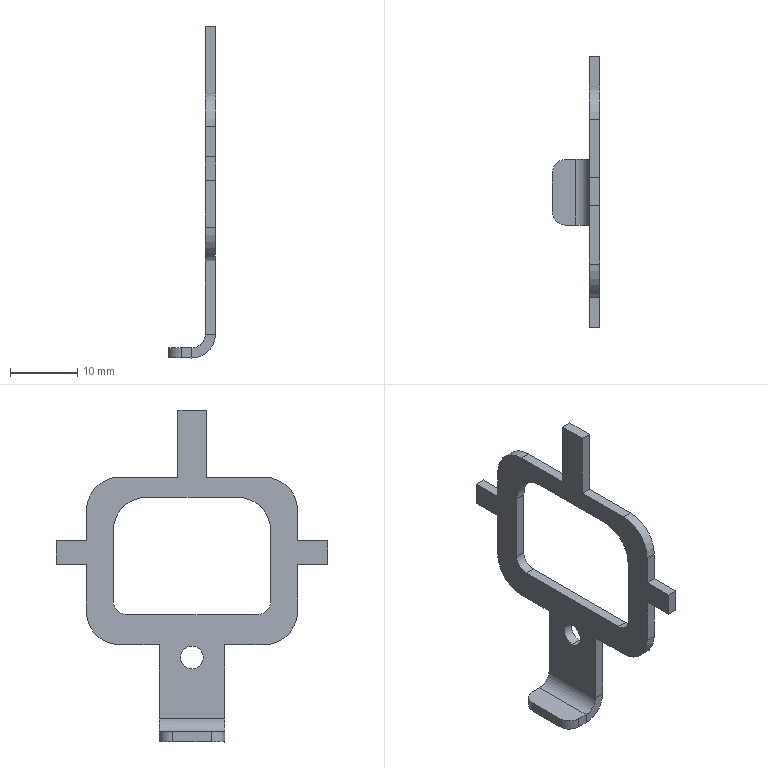Part | SolidWorks | features BaseBody 1 | 1 solid | 46 faces | box 7.041 x 40.502 x 49.501 mm | volume 921.56 mm3 | plane 32 | cylinder 14 | commonest cylinder face diameters 10 x6 4 x5 3.4 x2 7 x1
STEP:
#1=CARTESIAN_POINT('',(-263.159,-4.536,-94.753));
#2=VERTEX_POINT('',#1);
#3=CARTESIAN_POINT('',(-263.16,-4.535,-96.253));
#4=VERTEX_POINT('',#3);
#5=CARTESIAN_POINT('',(-263.159,-4.536,-94.753));
#6=DIRECTION('',(-0.0008339,0.0004454,-1.));
#7=VECTOR('',#6,1000.);
#8=LINE('',#5,#7);
#9=EDGE_CURVE('',#2,#4,#8,.T.);
#10=ORIENTED_EDGE('',*,*,#9,.F.);
#11=CARTESIAN_POINT('',(-261.159,-2.536,-94.754));
#12=VERTEX_POINT('',#11);
#13=CARTESIAN_POINT('',(-261.159,-4.536,-94.755));
#14=DIRECTION('',(-0.0008339,0.0004454,-1.));
#15=DIRECTION('',(-1.,-0.00003864,0.0008339));
#16=AXIS2_PLACEMENT_3D('',#13,#14,#15);
#17=CIRCLE('',#16,2.);
#18=EDGE_CURVE('',#2,#12,#17,.T.);
#19=ORIENTED_EDGE('',*,*,#18,.T.);
#20=CARTESIAN_POINT('',(-261.16,-2.535,-96.254));
#21=VERTEX_POINT('',#20);
#22=CARTESIAN_POINT('',(-261.16,-2.535,-96.254));
#23=DIRECTION('',(0.0008339,-0.0004454,1.));
#24=VECTOR('',#23,1000.);
#25=LINE('',#22,#24);
#26=EDGE_CURVE('',#21,#12,#25,.T.);
#27=ORIENTED_EDGE('',*,*,#26,.F.);
#28=CARTESIAN_POINT('',(-261.16,-4.535,-96.255));
#29=DIRECTION('',(0.0008339,-0.0004454,1.));
#30=DIRECTION('',(-0.00003827,1.,0.0004455));
#31=AXIS2_PLACEMENT_3D('',#28,#29,#30);
#32=CIRCLE('',#31,2.);
#33=EDGE_CURVE('',#21,#4,#32,.T.);
#34=ORIENTED_EDGE('',*,*,#33,.T.);
#35=EDGE_LOOP('',(#10,#19,#27,#34));
#36=FACE_OUTER_BOUND('',#35,.T.);
#37=CARTESIAN_POINT('',(-261.16,-4.535,-96.255));
#38=DIRECTION('',(0.0008339,-0.0004454,1.));
#39=DIRECTION('',(-1.,-0.00003864,0.0008339));
#40=AXIS2_PLACEMENT_3D('',#37,#38,#39);
#41=CYLINDRICAL_SURFACE('',#40,2.);
#42=ADVANCED_FACE('',(#36),#41,.T.);
#43=CARTESIAN_POINT('',(-263.16,-10.335,-96.256));
#44=VERTEX_POINT('',#43);
#45=CARTESIAN_POINT('',(-261.16,-12.335,-96.259));
#46=VERTEX_POINT('',#45);
#47=CARTESIAN_POINT('',(-261.16,-10.335,-96.258));
#48=DIRECTION('',(0.0008339,-0.0004454,1.));
#49=DIRECTION('',(-1.,-0.00003864,0.0008339));
#50=AXIS2_PLACEMENT_3D('',#47,#48,#49);
#51=CIRCLE('',#50,2.);
#52=EDGE_CURVE('',#44,#46,#51,.T.);
#53=ORIENTED_EDGE('',*,*,#52,.F.);
#54=CARTESIAN_POINT('',(-263.16,-4.535,-96.253));
#55=DIRECTION('',(0.00003827,-1.,-0.0004455));
#56=VECTOR('',#55,1000.);
#57=LINE('',#54,#56);
#58=EDGE_CURVE('',#4,#44,#57,.T.);
#59=ORIENTED_EDGE('',*,*,#58,.F.);
#60=ORIENTED_EDGE('',*,*,#33,.F.);
#61=CARTESIAN_POINT('',(-259.66,-2.535,-96.256));
#62=VERTEX_POINT('',#61);
#63=CARTESIAN_POINT('',(-259.66,-2.535,-96.256));
#64=DIRECTION('',(-1.,-0.00003864,0.0008339));
#65=VECTOR('',#64,1000.);
#66=LINE('',#63,#65);
#67=EDGE_CURVE('',#62,#21,#66,.T.);
#68=ORIENTED_EDGE('',*,*,#67,.F.);
#69=CARTESIAN_POINT('',(-259.66,-12.335,-96.26));
#70=VERTEX_POINT('',#69);
#71=CARTESIAN_POINT('',(-259.66,-2.535,-96.256));
#72=DIRECTION('',(0.00003827,-1.,-0.0004455));
#73=VECTOR('',#72,1000.);
#74=LINE('',#71,#73);
#75=EDGE_CURVE('',#62,#70,#74,.T.);
#76=ORIENTED_EDGE('',*,*,#75,.T.);
#77=CARTESIAN_POINT('',(-261.16,-12.335,-96.259));
#78=DIRECTION('',(1.,0.00003864,-0.0008339));
#79=VECTOR('',#78,1000.);
#80=LINE('',#77,#79);
#81=EDGE_CURVE('',#46,#70,#80,.T.);
#82=ORIENTED_EDGE('',*,*,#81,.F.);
#83=EDGE_LOOP('',(#53,#59,#60,#68,#76,#82));
#84=FACE_OUTER_BOUND('',#83,.T.);
#85=CARTESIAN_POINT('',(-257.661,8.315,-96.252));
#86=DIRECTION('',(0.0008339,-0.0004454,1.));
#87=DIRECTION('',(-0.4711,-0.8821,0.));
#88=AXIS2_PLACEMENT_3D('',#85,#86,#87);
#89=PLANE('',#88);
#90=ADVANCED_FACE('',(#84),#89,.F.);
#91=CARTESIAN_POINT('',(-261.159,-12.336,-94.759));
#92=VERTEX_POINT('',#91);
#93=CARTESIAN_POINT('',(-261.159,-12.336,-94.759));
#94=DIRECTION('',(-0.0008339,0.0004454,-1.));
#95=VECTOR('',#94,1000.);
#96=LINE('',#93,#95);
#97=EDGE_CURVE('',#92,#46,#96,.T.);
#98=ORIENTED_EDGE('',*,*,#97,.T.);
#99=ORIENTED_EDGE('',*,*,#81,.T.);
#100=CARTESIAN_POINT('',(-259.659,-12.336,-94.76));
#101=VERTEX_POINT('',#100);
#102=CARTESIAN_POINT('',(-259.66,-12.335,-96.26));
#103=DIRECTION('',(0.0008339,-0.0004454,1.));
#104=VECTOR('',#103,1000.);
#105=LINE('',#102,#104);
#106=EDGE_CURVE('',#70,#101,#105,.T.);
#107=ORIENTED_EDGE('',*,*,#106,.T.);
#108=CARTESIAN_POINT('',(-261.159,-12.336,-94.759));
#109=DIRECTION('',(1.,0.00003864,-0.0008339));
#110=VECTOR('',#109,1000.);
#111=LINE('',#108,#110);
#112=EDGE_CURVE('',#92,#101,#111,.T.);
#113=ORIENTED_EDGE('',*,*,#112,.F.);
#114=EDGE_LOOP('',(#98,#99,#107,#113));
#115=FACE_OUTER_BOUND('',#114,.T.);
#116=CARTESIAN_POINT('',(-263.16,-12.335,-96.257));
#117=DIRECTION('',(-0.00003827,1.,0.0004455));
#118=DIRECTION('',(0.9963,0.,0.08559));
#119=AXIS2_PLACEMENT_3D('',#116,#117,#118);
#120=PLANE('',#119);
#121=ADVANCED_FACE('',(#115),#120,.F.);
#122=CARTESIAN_POINT('',(-263.159,-10.336,-94.756));
#123=VERTEX_POINT('',#122);
#124=CARTESIAN_POINT('',(-261.159,-10.336,-94.758));
#125=DIRECTION('',(-0.0008339,0.0004454,-1.));
#126=DIRECTION('',(0.00003827,-1.,-0.0004455));
#127=AXIS2_PLACEMENT_3D('',#124,#125,#126);
#128=CIRCLE('',#127,2.);
#129=EDGE_CURVE('',#92,#123,#128,.T.);
#130=ORIENTED_EDGE('',*,*,#129,.F.);
#131=ORIENTED_EDGE('',*,*,#112,.T.);
#132=CARTESIAN_POINT('',(-259.659,-2.536,-94.756));
#133=VERTEX_POINT('',#132);
#134=CARTESIAN_POINT('',(-259.659,-12.336,-94.76));
#135=DIRECTION('',(-0.00003827,1.,0.0004455));
#136=VECTOR('',#135,1000.);
#137=LINE('',#134,#136);
#138=EDGE_CURVE('',#101,#133,#137,.T.);
#139=ORIENTED_EDGE('',*,*,#138,.T.);
#140=CARTESIAN_POINT('',(-259.659,-2.536,-94.756));
#141=DIRECTION('',(-1.,-0.00003864,0.0008339));
#142=VECTOR('',#141,1000.);
#143=LINE('',#140,#142);
#144=EDGE_CURVE('',#133,#12,#143,.T.);
#145=ORIENTED_EDGE('',*,*,#144,.T.);
#146=ORIENTED_EDGE('',*,*,#18,.F.);
#147=CARTESIAN_POINT('',(-263.159,-4.536,-94.753));
#148=DIRECTION('',(0.00003827,-1.,-0.0004455));
#149=VECTOR('',#148,1000.);
#150=LINE('',#147,#149);
#151=EDGE_CURVE('',#2,#123,#150,.T.);
#152=ORIENTED_EDGE('',*,*,#151,.T.);
#153=EDGE_LOOP('',(#130,#131,#139,#145,#146,#152));
#154=FACE_OUTER_BOUND('',#153,.T.);
#155=CARTESIAN_POINT('',(-257.66,8.314,-94.752));
#156=DIRECTION('',(0.0008339,-0.0004454,1.));
#157=DIRECTION('',(-0.4711,-0.8821,0.));
#158=AXIS2_PLACEMENT_3D('',#155,#156,#157);
#159=PLANE('',#158);
#160=ADVANCED_FACE('',(#154),#159,.T.);
#161=CARTESIAN_POINT('',(-263.16,-10.335,-96.256));
#162=DIRECTION('',(0.0008339,-0.0004454,1.));
#163=VECTOR('',#162,1000.);
#164=LINE('',#161,#163);
#165=EDGE_CURVE('',#44,#123,#164,.T.);
#166=ORIENTED_EDGE('',*,*,#165,.T.);
#167=ORIENTED_EDGE('',*,*,#151,.F.);
#168=ORIENTED_EDGE('',*,*,#9,.T.);
#169=ORIENTED_EDGE('',*,*,#58,.T.);
#170=EDGE_LOOP('',(#166,#167,#168,#169));
#171=FACE_OUTER_BOUND('',#170,.T.);
#172=CARTESIAN_POINT('',(-263.16,-2.535,-96.253));
#173=DIRECTION('',(1.,0.00003864,-0.0008339));
#174=DIRECTION('',(0.,-0.9989,-0.04628));
#175=AXIS2_PLACEMENT_3D('',#172,#173,#174);
#176=PLANE('',#175);
#177=ADVANCED_FACE('',(#171),#176,.F.);
#178=ORIENTED_EDGE('',*,*,#97,.F.);
#179=ORIENTED_EDGE('',*,*,#129,.T.);
#180=ORIENTED_EDGE('',*,*,#165,.F.);
#181=ORIENTED_EDGE('',*,*,#52,.T.);
#182=EDGE_LOOP('',(#178,#179,#180,#181));
#183=FACE_OUTER_BOUND('',#182,.T.);
#184=CARTESIAN_POINT('',(-261.16,-10.335,-96.258));
#185=DIRECTION('',(0.0008339,-0.0004454,1.));
#186=DIRECTION('',(-1.,-0.00003864,0.0008339));
#187=AXIS2_PLACEMENT_3D('',#184,#185,#186);
#188=CYLINDRICAL_SURFACE('',#187,2.);
#189=ADVANCED_FACE('',(#183),#188,.T.);
#190=ORIENTED_EDGE('',*,*,#26,.T.);
#191=ORIENTED_EDGE('',*,*,#144,.F.);
#192=CARTESIAN_POINT('',(-259.66,-2.535,-96.256));
#193=DIRECTION('',(0.0008339,-0.0004454,1.));
#194=VECTOR('',#193,1000.);
#195=LINE('',#192,#194);
#196=EDGE_CURVE('',#62,#133,#195,.T.);
#197=ORIENTED_EDGE('',*,*,#196,.F.);
#198=ORIENTED_EDGE('',*,*,#67,.T.);
#199=EDGE_LOOP('',(#190,#191,#197,#198));
#200=FACE_OUTER_BOUND('',#199,.T.);
#201=CARTESIAN_POINT('',(-257.66,-2.535,-96.257));
#202=DIRECTION('',(0.00003827,-1.,-0.0004455));
#203=DIRECTION('',(0.,0.0004455,-1.));
#204=AXIS2_PLACEMENT_3D('',#201,#202,#203);
#205=PLANE('',#204);
#206=ADVANCED_FACE('',(#200),#205,.F.);
#207=CARTESIAN_POINT('',(-257.657,-2.537,-92.757));
#208=VERTEX_POINT('',#207);
#209=CARTESIAN_POINT('',(-259.657,-2.537,-92.756));
#210=DIRECTION('',(-0.00003827,1.,0.0004455));
#211=DIRECTION('',(1.,0.00003864,-0.0008339));
#212=AXIS2_PLACEMENT_3D('',#209,#210,#211);
#213=CIRCLE('',#212,2.);
#214=EDGE_CURVE('',#208,#133,#213,.T.);
#215=ORIENTED_EDGE('',*,*,#214,.F.);
#216=CARTESIAN_POINT('',(-256.157,-2.537,-92.758));
#217=VERTEX_POINT('',#216);
#218=CARTESIAN_POINT('',(-256.157,-2.537,-92.758));
#219=DIRECTION('',(-1.,-0.00003864,0.0008339));
#220=VECTOR('',#219,1000.);
#221=LINE('',#218,#220);
#222=EDGE_CURVE('',#217,#208,#221,.T.);
#223=ORIENTED_EDGE('',*,*,#222,.F.);
#224=CARTESIAN_POINT('',(-259.657,-2.537,-92.756));
#225=DIRECTION('',(0.00003827,-1.,-0.0004455));
#226=DIRECTION('',(-0.0008339,0.0004454,-1.));
#227=AXIS2_PLACEMENT_3D('',#224,#225,#226);
#228=CIRCLE('',#227,3.5);
#229=EDGE_CURVE('',#62,#217,#228,.T.);
#230=ORIENTED_EDGE('',*,*,#229,.F.);
#231=ORIENTED_EDGE('',*,*,#196,.T.);
#232=EDGE_LOOP('',(#215,#223,#230,#231));
#233=FACE_OUTER_BOUND('',#232,.T.);
#234=CARTESIAN_POINT('',(-259.657,-2.537,-92.756));
#235=DIRECTION('',(-0.00003827,1.,0.0004455));
#236=DIRECTION('',(0.9963,0.,0.08559));
#237=AXIS2_PLACEMENT_3D('',#234,#235,#236);
#238=PLANE('',#237);
#239=ADVANCED_FACE('',(#233),#238,.T.);
#240=CARTESIAN_POINT('',(-256.157,-12.337,-92.763));
#241=VERTEX_POINT('',#240);
#242=CARTESIAN_POINT('',(-259.657,-12.337,-92.76));
#243=DIRECTION('',(-0.00003827,1.,0.0004455));
#244=DIRECTION('',(1.,0.00003864,-0.0008339));
#245=AXIS2_PLACEMENT_3D('',#242,#243,#244);
#246=CIRCLE('',#245,3.5);
#247=EDGE_CURVE('',#241,#70,#246,.T.);
#248=ORIENTED_EDGE('',*,*,#247,.T.);
#249=ORIENTED_EDGE('',*,*,#75,.F.);
#250=ORIENTED_EDGE('',*,*,#229,.T.);
#251=CARTESIAN_POINT('',(-256.157,-12.337,-92.763));
#252=DIRECTION('',(-0.00003827,1.,0.0004455));
#253=VECTOR('',#252,1000.);
#254=LINE('',#251,#253);
#255=EDGE_CURVE('',#241,#217,#254,.T.);
#256=ORIENTED_EDGE('',*,*,#255,.F.);
#257=EDGE_LOOP('',(#248,#249,#250,#256));
#258=FACE_OUTER_BOUND('',#257,.T.);
#259=CARTESIAN_POINT('',(-259.657,-12.337,-92.76));
#260=DIRECTION('',(0.00003827,-1.,-0.0004455));
#261=DIRECTION('',(-0.0008339,0.0004454,-1.));
#262=AXIS2_PLACEMENT_3D('',#259,#260,#261);
#263=CYLINDRICAL_SURFACE('',#262,3.5);
#264=ADVANCED_FACE('',(#258),#263,.T.);
#265=CARTESIAN_POINT('',(-256.142,-19.194,-75.266));
#266=VERTEX_POINT('',#265);
#267=CARTESIAN_POINT('',(-256.144,-17.193,-77.265));
#268=VERTEX_POINT('',#267);
#269=CARTESIAN_POINT('',(-256.142,-17.194,-75.265));
#270=DIRECTION('',(1.,0.00003864,-0.0008339));
#271=DIRECTION('',(0.00003827,-1.,-0.0004455));
#272=AXIS2_PLACEMENT_3D('',#269,#270,#271);
#273=CIRCLE('',#272,2.);
#274=EDGE_CURVE('',#266,#268,#273,.T.);
#275=ORIENTED_EDGE('',*,*,#274,.F.);
#276=CARTESIAN_POINT('',(-256.133,-19.199,-64.766));
#277=VERTEX_POINT('',#276);
#278=CARTESIAN_POINT('',(-256.133,-19.199,-64.766));
#279=DIRECTION('',(-0.0008339,0.0004454,-1.));
#280=VECTOR('',#279,1000.);
#281=LINE('',#278,#280);
#282=EDGE_CURVE('',#277,#266,#281,.T.);
#283=ORIENTED_EDGE('',*,*,#282,.F.);
#284=CARTESIAN_POINT('',(-256.129,-14.201,-59.764));
#285=VERTEX_POINT('',#284);
#286=CARTESIAN_POINT('',(-256.134,-14.199,-64.764));
#287=DIRECTION('',(1.,0.00003864,-0.0008339));
#288=DIRECTION('',(0.0008339,-0.0004454,1.));
#289=AXIS2_PLACEMENT_3D('',#286,#287,#288);
#290=CIRCLE('',#289,5.);
#291=EDGE_CURVE('',#285,#277,#290,.T.);
#292=ORIENTED_EDGE('',*,*,#291,.F.);
#293=CARTESIAN_POINT('',(-256.13,-0.7013,-59.758));
#294=VERTEX_POINT('',#293);
#295=CARTESIAN_POINT('',(-256.13,-0.7013,-59.758));
#296=DIRECTION('',(0.00003827,-1.,-0.0004455));
#297=VECTOR('',#296,1000.);
#298=LINE('',#295,#297);
#299=EDGE_CURVE('',#294,#285,#298,.T.);
#300=ORIENTED_EDGE('',*,*,#299,.F.);
#301=CARTESIAN_POINT('',(-256.134,4.301,-64.755));
#302=VERTEX_POINT('',#301);
#303=CARTESIAN_POINT('',(-256.134,-0.699,-64.758));
#304=DIRECTION('',(1.,0.00003864,-0.0008339));
#305=DIRECTION('',(-0.00003827,1.,0.0004455));
#306=AXIS2_PLACEMENT_3D('',#303,#304,#305);
#307=CIRCLE('',#306,5.);
#308=EDGE_CURVE('',#302,#294,#307,.T.);
#309=ORIENTED_EDGE('',*,*,#308,.F.);
#310=CARTESIAN_POINT('',(-256.143,4.306,-75.255));
#311=VERTEX_POINT('',#310);
#312=CARTESIAN_POINT('',(-256.143,4.306,-75.255));
#313=DIRECTION('',(0.0008339,-0.0004454,1.));
#314=VECTOR('',#313,1000.);
#315=LINE('',#312,#314);
#316=EDGE_CURVE('',#311,#302,#315,.T.);
#317=ORIENTED_EDGE('',*,*,#316,.F.);
#318=CARTESIAN_POINT('',(-256.145,2.307,-77.256));
#319=VERTEX_POINT('',#318);
#320=CARTESIAN_POINT('',(-256.143,2.306,-75.256));
#321=DIRECTION('',(1.,0.00003864,-0.0008339));
#322=DIRECTION('',(-0.0008339,0.0004454,-1.));
#323=AXIS2_PLACEMENT_3D('',#320,#321,#322);
#324=CIRCLE('',#323,2.);
#325=EDGE_CURVE('',#319,#311,#324,.T.);
#326=ORIENTED_EDGE('',*,*,#325,.F.);
#327=CARTESIAN_POINT('',(-256.144,-17.193,-77.265));
#328=DIRECTION('',(-0.00003827,1.,0.0004455));
#329=VECTOR('',#328,1000.);
#330=LINE('',#327,#329);
#331=EDGE_CURVE('',#268,#319,#330,.T.);
#332=ORIENTED_EDGE('',*,*,#331,.F.);
#333=EDGE_LOOP('',(#275,#283,#292,#300,#309,#317,#326,#332));
#334=FACE_BOUND('',#333,.T.);
#335=CARTESIAN_POINT('',(-256.148,-7.441,-81.961));
#336=VERTEX_POINT('',#335);
#337=CARTESIAN_POINT('',(-256.151,-7.44,-85.361));
#338=VERTEX_POINT('',#337);
#339=CARTESIAN_POINT('',(-256.15,-7.441,-83.661));
#340=DIRECTION('',(1.,0.00003864,-0.0008339));
#341=DIRECTION('',(0.0008339,-0.0004454,1.));
#342=AXIS2_PLACEMENT_3D('',#339,#340,#341);
#343=CIRCLE('',#342,1.7);
#344=EDGE_CURVE('',#336,#338,#343,.T.);
#345=ORIENTED_EDGE('',*,*,#344,.F.);
#346=CARTESIAN_POINT('',(-256.15,-7.441,-83.661));
#347=DIRECTION('',(1.,0.00003864,-0.0008339));
#348=DIRECTION('',(-0.0008339,0.0004454,-1.));
#349=AXIS2_PLACEMENT_3D('',#346,#347,#348);
#350=CIRCLE('',#349,1.7);
#351=EDGE_CURVE('',#338,#336,#350,.T.);
#352=ORIENTED_EDGE('',*,*,#351,.F.);
#353=EDGE_LOOP('',(#345,#352));
#354=FACE_BOUND('',#353,.T.);
#355=ORIENTED_EDGE('',*,*,#255,.T.);
#356=CARTESIAN_POINT('',(-256.148,-2.541,-81.758));
#357=VERTEX_POINT('',#356);
#358=CARTESIAN_POINT('',(-256.157,-2.537,-92.758));
#359=DIRECTION('',(0.0008339,-0.0004454,1.));
#360=VECTOR('',#359,1000.);
#361=LINE('',#358,#360);
#362=EDGE_CURVE('',#217,#357,#361,.T.);
#363=ORIENTED_EDGE('',*,*,#362,.T.);
#364=CARTESIAN_POINT('',(-256.148,3.309,-81.756));
#365=VERTEX_POINT('',#364);
#366=CARTESIAN_POINT('',(-256.148,-2.541,-81.758));
#367=DIRECTION('',(-0.00003827,1.,0.0004455));
#368=VECTOR('',#367,1000.);
#369=LINE('',#366,#368);
#370=EDGE_CURVE('',#357,#365,#369,.T.);
#371=ORIENTED_EDGE('',*,*,#370,.T.);
#372=CARTESIAN_POINT('',(-256.145,8.306,-76.754));
#373=VERTEX_POINT('',#372);
#374=CARTESIAN_POINT('',(-256.144,3.306,-76.756));
#375=DIRECTION('',(-1.,-0.00003864,0.0008339));
#376=DIRECTION('',(-0.00003827,1.,0.0004455));
#377=AXIS2_PLACEMENT_3D('',#374,#375,#376);
#378=CIRCLE('',#377,5.);
#379=EDGE_CURVE('',#373,#365,#378,.T.);
#380=ORIENTED_EDGE('',*,*,#379,.F.);
#381=CARTESIAN_POINT('',(-256.139,8.303,-69.754));
#382=VERTEX_POINT('',#381);
#383=CARTESIAN_POINT('',(-256.145,8.306,-76.754));
#384=DIRECTION('',(0.0008339,-0.0004454,1.));
#385=VECTOR('',#384,1000.);
#386=LINE('',#383,#385);
#387=EDGE_CURVE('',#373,#382,#386,.T.);
#388=ORIENTED_EDGE('',*,*,#387,.T.);
#389=CARTESIAN_POINT('',(-256.139,12.803,-69.752));
#390=VERTEX_POINT('',#389);
#391=CARTESIAN_POINT('',(-256.139,8.303,-69.754));
#392=DIRECTION('',(-0.00003827,1.,0.0004455));
#393=VECTOR('',#392,1000.);
#394=LINE('',#391,#393);
#395=EDGE_CURVE('',#382,#390,#394,.T.);
#396=ORIENTED_EDGE('',*,*,#395,.T.);
#397=CARTESIAN_POINT('',(-256.136,12.802,-66.252));
#398=VERTEX_POINT('',#397);
#399=CARTESIAN_POINT('',(-256.139,12.803,-69.752));
#400=DIRECTION('',(0.0008339,-0.0004454,1.));
#401=VECTOR('',#400,1000.);
#402=LINE('',#399,#401);
#403=EDGE_CURVE('',#390,#398,#402,.T.);
#404=ORIENTED_EDGE('',*,*,#403,.T.);
#405=CARTESIAN_POINT('',(-256.136,8.302,-66.254));
#406=VERTEX_POINT('',#405);
#407=CARTESIAN_POINT('',(-256.136,12.802,-66.252));
#408=DIRECTION('',(0.00003827,-1.,-0.0004455));
#409=VECTOR('',#408,1000.);
#410=LINE('',#407,#409);
#411=EDGE_CURVE('',#398,#406,#410,.T.);
#412=ORIENTED_EDGE('',*,*,#411,.T.);
#413=CARTESIAN_POINT('',(-256.132,8.3,-61.754));
#414=VERTEX_POINT('',#413);
#415=CARTESIAN_POINT('',(-256.136,8.302,-66.254));
#416=DIRECTION('',(0.0008339,-0.0004454,1.));
#417=VECTOR('',#416,1000.);
#418=LINE('',#415,#417);
#419=EDGE_CURVE('',#406,#414,#418,.T.);
#420=ORIENTED_EDGE('',*,*,#419,.T.);
#421=CARTESIAN_POINT('',(-256.128,3.297,-56.756));
#422=VERTEX_POINT('',#421);
#423=CARTESIAN_POINT('',(-256.132,3.3,-61.756));
#424=DIRECTION('',(-1.,-0.00003864,0.0008339));
#425=DIRECTION('',(0.0008339,-0.0004454,1.));
#426=AXIS2_PLACEMENT_3D('',#423,#424,#425);
#427=CIRCLE('',#426,5.);
#428=EDGE_CURVE('',#422,#414,#427,.T.);
#429=ORIENTED_EDGE('',*,*,#428,.F.);
#430=CARTESIAN_POINT('',(-256.127,-5.353,-56.76));
#431=VERTEX_POINT('',#430);
#432=CARTESIAN_POINT('',(-256.128,3.297,-56.756));
#433=DIRECTION('',(0.00003827,-1.,-0.0004455));
#434=VECTOR('',#433,1000.);
#435=LINE('',#432,#434);
#436=EDGE_CURVE('',#422,#431,#435,.T.);
#437=ORIENTED_EDGE('',*,*,#436,.T.);
#438=CARTESIAN_POINT('',(-256.119,-5.357,-46.76));
#439=VERTEX_POINT('',#438);
#440=CARTESIAN_POINT('',(-256.127,-5.353,-56.76));
#441=DIRECTION('',(0.0008339,-0.0004454,1.));
#442=VECTOR('',#441,1000.);
#443=LINE('',#440,#442);
#444=EDGE_CURVE('',#431,#439,#443,.T.);
#445=ORIENTED_EDGE('',*,*,#444,.T.);
#446=CARTESIAN_POINT('',(-256.119,-9.557,-46.762));
#447=VERTEX_POINT('',#446);
#448=CARTESIAN_POINT('',(-256.119,-5.357,-46.76));
#449=DIRECTION('',(0.00003827,-1.,-0.0004455));
#450=VECTOR('',#449,1000.);
#451=LINE('',#448,#450);
#452=EDGE_CURVE('',#439,#447,#451,.T.);
#453=ORIENTED_EDGE('',*,*,#452,.T.);
#454=CARTESIAN_POINT('',(-256.127,-9.553,-56.762));
#455=VERTEX_POINT('',#454);
#456=CARTESIAN_POINT('',(-256.119,-9.557,-46.762));
#457=DIRECTION('',(-0.0008339,0.0004454,-1.));
#458=VECTOR('',#457,1000.);
#459=LINE('',#456,#458);
#460=EDGE_CURVE('',#447,#455,#459,.T.);
#461=ORIENTED_EDGE('',*,*,#460,.T.);
#462=CARTESIAN_POINT('',(-256.127,-18.203,-56.765));
#463=VERTEX_POINT('',#462);
#464=CARTESIAN_POINT('',(-256.127,-9.553,-56.762));
#465=DIRECTION('',(0.00003827,-1.,-0.0004455));
#466=VECTOR('',#465,1000.);
#467=LINE('',#464,#466);
#468=EDGE_CURVE('',#455,#463,#467,.T.);
#469=ORIENTED_EDGE('',*,*,#468,.T.);
#470=CARTESIAN_POINT('',(-256.131,-23.2,-61.768));
#471=VERTEX_POINT('',#470);
#472=CARTESIAN_POINT('',(-256.131,-18.2,-61.765));
#473=DIRECTION('',(-1.,-0.00003864,0.0008339));
#474=DIRECTION('',(0.00003827,-1.,-0.0004455));
#475=AXIS2_PLACEMENT_3D('',#472,#473,#474);
#476=CIRCLE('',#475,5.);
#477=EDGE_CURVE('',#471,#463,#476,.T.);
#478=ORIENTED_EDGE('',*,*,#477,.F.);
#479=CARTESIAN_POINT('',(-256.135,-23.198,-66.268));
#480=VERTEX_POINT('',#479);
#481=CARTESIAN_POINT('',(-256.131,-23.2,-61.768));
#482=DIRECTION('',(-0.0008339,0.0004454,-1.));
#483=VECTOR('',#482,1000.);
#484=LINE('',#481,#483);
#485=EDGE_CURVE('',#471,#480,#484,.T.);
#486=ORIENTED_EDGE('',*,*,#485,.T.);
#487=CARTESIAN_POINT('',(-256.134,-27.698,-66.27));
#488=VERTEX_POINT('',#487);
#489=CARTESIAN_POINT('',(-256.135,-23.198,-66.268));
#490=DIRECTION('',(0.00003827,-1.,-0.0004455));
#491=VECTOR('',#490,1000.);
#492=LINE('',#489,#491);
#493=EDGE_CURVE('',#480,#488,#492,.T.);
#494=ORIENTED_EDGE('',*,*,#493,.T.);
#495=CARTESIAN_POINT('',(-256.137,-27.697,-69.77));
#496=VERTEX_POINT('',#495);
#497=CARTESIAN_POINT('',(-256.134,-27.698,-66.27));
#498=DIRECTION('',(-0.0008339,0.0004454,-1.));
#499=VECTOR('',#498,1000.);
#500=LINE('',#497,#499);
#501=EDGE_CURVE('',#488,#496,#500,.T.);
#502=ORIENTED_EDGE('',*,*,#501,.T.);
#503=CARTESIAN_POINT('',(-256.137,-23.197,-69.768));
#504=VERTEX_POINT('',#503);
#505=CARTESIAN_POINT('',(-256.137,-27.697,-69.77));
#506=DIRECTION('',(-0.00003827,1.,0.0004455));
#507=VECTOR('',#506,1000.);
#508=LINE('',#505,#507);
#509=EDGE_CURVE('',#496,#504,#508,.T.);
#510=ORIENTED_EDGE('',*,*,#509,.T.);
#511=CARTESIAN_POINT('',(-256.143,-23.194,-76.768));
#512=VERTEX_POINT('',#511);
#513=CARTESIAN_POINT('',(-256.137,-23.197,-69.768));
#514=DIRECTION('',(-0.0008339,0.0004454,-1.));
#515=VECTOR('',#514,1000.);
#516=LINE('',#513,#515);
#517=EDGE_CURVE('',#504,#512,#516,.T.);
#518=ORIENTED_EDGE('',*,*,#517,.T.);
#519=CARTESIAN_POINT('',(-256.148,-18.191,-81.765));
#520=VERTEX_POINT('',#519);
#521=CARTESIAN_POINT('',(-256.143,-18.194,-76.765));
#522=DIRECTION('',(-1.,-0.00003864,0.0008339));
#523=DIRECTION('',(-0.0008339,0.0004454,-1.));
#524=AXIS2_PLACEMENT_3D('',#521,#522,#523);
#525=CIRCLE('',#524,5.);
#526=EDGE_CURVE('',#520,#512,#525,.T.);
#527=ORIENTED_EDGE('',*,*,#526,.F.);
#528=CARTESIAN_POINT('',(-256.148,-12.341,-81.763));
#529=VERTEX_POINT('',#528);
#530=CARTESIAN_POINT('',(-256.148,-18.191,-81.765));
#531=DIRECTION('',(-0.00003827,1.,0.0004455));
#532=VECTOR('',#531,1000.);
#533=LINE('',#530,#532);
#534=EDGE_CURVE('',#520,#529,#533,.T.);
#535=ORIENTED_EDGE('',*,*,#534,.T.);
#536=CARTESIAN_POINT('',(-256.148,-12.341,-81.763));
#537=DIRECTION('',(-0.0008339,0.0004454,-1.));
#538=VECTOR('',#537,1000.);
#539=LINE('',#536,#538);
#540=EDGE_CURVE('',#529,#241,#539,.T.);
#541=ORIENTED_EDGE('',*,*,#540,.T.);
#542=EDGE_LOOP('',(#355,#363,#371,#380,#388,#396,#404,#412,#420,#429,#437,#445,#453,#461,#469,#478,#486,#494,#502,#510,#518,#527,#535,#541));
#543=FACE_OUTER_BOUND('',#542,.T.);
#544=CARTESIAN_POINT('',(-256.128,8.297,-56.754));
#545=DIRECTION('',(1.,0.00003864,-0.0008339));
#546=DIRECTION('',(0.,-0.9989,-0.04628));
#547=AXIS2_PLACEMENT_3D('',#544,#545,#546);
#548=PLANE('',#547);
#549=ADVANCED_FACE('',(#334,#354,#543),#548,.T.);
#550=CARTESIAN_POINT('',(-257.657,-12.337,-92.762));
#551=VERTEX_POINT('',#550);
#552=CARTESIAN_POINT('',(-256.157,-12.337,-92.763));
#553=DIRECTION('',(-1.,-0.00003864,0.0008339));
#554=VECTOR('',#553,1000.);
#555=LINE('',#552,#554);
#556=EDGE_CURVE('',#241,#551,#555,.T.);
#557=ORIENTED_EDGE('',*,*,#556,.F.);
#558=ORIENTED_EDGE('',*,*,#540,.F.);
#559=CARTESIAN_POINT('',(-257.648,-12.342,-81.762));
#560=VERTEX_POINT('',#559);
#561=CARTESIAN_POINT('',(-257.648,-12.342,-81.762));
#562=DIRECTION('',(1.,0.00003864,-0.0008339));
#563=VECTOR('',#562,1000.);
#564=LINE('',#561,#563);
#565=EDGE_CURVE('',#560,#529,#564,.T.);
#566=ORIENTED_EDGE('',*,*,#565,.F.);
#567=CARTESIAN_POINT('',(-257.648,-12.342,-81.762));
#568=DIRECTION('',(-0.0008339,0.0004454,-1.));
#569=VECTOR('',#568,1000.);
#570=LINE('',#567,#569);
#571=EDGE_CURVE('',#560,#551,#570,.T.);
#572=ORIENTED_EDGE('',*,*,#571,.T.);
#573=EDGE_LOOP('',(#557,#558,#566,#572));
#574=FACE_OUTER_BOUND('',#573,.T.);
#575=CARTESIAN_POINT('',(-256.148,-12.341,-81.763));
#576=DIRECTION('',(0.00003827,-1.,-0.0004455));
#577=DIRECTION('',(0.,0.0004455,-1.));
#578=AXIS2_PLACEMENT_3D('',#575,#576,#577);
#579=PLANE('',#578);
#580=ADVANCED_FACE('',(#574),#579,.T.);
#581=CARTESIAN_POINT('',(-257.63,-0.7013,-59.756));
#582=VERTEX_POINT('',#581);
#583=CARTESIAN_POINT('',(-257.634,4.301,-64.754));
#584=VERTEX_POINT('',#583);
#585=CARTESIAN_POINT('',(-257.634,-0.6991,-64.756));
#586=DIRECTION('',(-1.,-0.00003864,0.0008339));
#587=DIRECTION('',(0.0008339,-0.0004454,1.));
#588=AXIS2_PLACEMENT_3D('',#585,#586,#587);
#589=CIRCLE('',#588,5.);
#590=EDGE_CURVE('',#582,#584,#589,.T.);
#591=ORIENTED_EDGE('',*,*,#590,.F.);
#592=CARTESIAN_POINT('',(-257.629,-14.201,-59.762));
#593=VERTEX_POINT('',#592);
#594=CARTESIAN_POINT('',(-257.63,-0.7013,-59.756));
#595=DIRECTION('',(0.00003827,-1.,-0.0004455));
#596=VECTOR('',#595,1000.);
#597=LINE('',#594,#596);
#598=EDGE_CURVE('',#582,#593,#597,.T.);
#599=ORIENTED_EDGE('',*,*,#598,.T.);
#600=CARTESIAN_POINT('',(-257.633,-19.199,-64.765));
#601=VERTEX_POINT('',#600);
#602=CARTESIAN_POINT('',(-257.634,-14.199,-64.762));
#603=DIRECTION('',(-1.,-0.00003864,0.0008339));
#604=DIRECTION('',(0.00003827,-1.,-0.0004455));
#605=AXIS2_PLACEMENT_3D('',#602,#603,#604);
#606=CIRCLE('',#605,5.);
#607=EDGE_CURVE('',#601,#593,#606,.T.);
#608=ORIENTED_EDGE('',*,*,#607,.F.);
#609=CARTESIAN_POINT('',(-257.642,-19.194,-75.265));
#610=VERTEX_POINT('',#609);
#611=CARTESIAN_POINT('',(-257.633,-19.199,-64.765));
#612=DIRECTION('',(-0.0008339,0.0004454,-1.));
#613=VECTOR('',#612,1000.);
#614=LINE('',#611,#613);
#615=EDGE_CURVE('',#601,#610,#614,.T.);
#616=ORIENTED_EDGE('',*,*,#615,.T.);
#617=CARTESIAN_POINT('',(-257.644,-17.194,-77.264));
#618=VERTEX_POINT('',#617);
#619=CARTESIAN_POINT('',(-257.642,-17.194,-75.264));
#620=DIRECTION('',(-1.,-0.00003864,0.0008339));
#621=DIRECTION('',(-0.0008339,0.0004454,-1.));
#622=AXIS2_PLACEMENT_3D('',#619,#620,#621);
#623=CIRCLE('',#622,2.);
#624=EDGE_CURVE('',#618,#610,#623,.T.);
#625=ORIENTED_EDGE('',*,*,#624,.F.);
#626=CARTESIAN_POINT('',(-257.645,2.306,-77.255));
#627=VERTEX_POINT('',#626);
#628=CARTESIAN_POINT('',(-257.644,-17.194,-77.264));
#629=DIRECTION('',(-0.00003827,1.,0.0004455));
#630=VECTOR('',#629,1000.);
#631=LINE('',#628,#630);
#632=EDGE_CURVE('',#618,#627,#631,.T.);
#633=ORIENTED_EDGE('',*,*,#632,.T.);
#634=CARTESIAN_POINT('',(-257.643,4.306,-75.254));
#635=VERTEX_POINT('',#634);
#636=CARTESIAN_POINT('',(-257.643,2.306,-75.255));
#637=DIRECTION('',(-1.,-0.00003864,0.0008339));
#638=DIRECTION('',(-0.00003827,1.,0.0004455));
#639=AXIS2_PLACEMENT_3D('',#636,#637,#638);
#640=CIRCLE('',#639,2.);
#641=EDGE_CURVE('',#635,#627,#640,.T.);
#642=ORIENTED_EDGE('',*,*,#641,.F.);
#643=CARTESIAN_POINT('',(-257.643,4.306,-75.254));
#644=DIRECTION('',(0.0008339,-0.0004454,1.));
#645=VECTOR('',#644,1000.);
#646=LINE('',#643,#645);
#647=EDGE_CURVE('',#635,#584,#646,.T.);
#648=ORIENTED_EDGE('',*,*,#647,.T.);
#649=EDGE_LOOP('',(#591,#599,#608,#616,#625,#633,#642,#648));
#650=FACE_BOUND('',#649,.T.);
#651=CARTESIAN_POINT('',(-257.648,-7.441,-81.959));
#652=VERTEX_POINT('',#651);
#653=CARTESIAN_POINT('',(-257.651,-7.44,-85.359));
#654=VERTEX_POINT('',#653);
#655=CARTESIAN_POINT('',(-257.65,-7.441,-83.659));
#656=DIRECTION('',(-1.,-0.00003864,0.0008339));
#657=DIRECTION('',(0.0008339,-0.0004454,1.));
#658=AXIS2_PLACEMENT_3D('',#655,#656,#657);
#659=CIRCLE('',#658,1.7);
#660=EDGE_CURVE('',#652,#654,#659,.T.);
#661=ORIENTED_EDGE('',*,*,#660,.F.);
#662=CARTESIAN_POINT('',(-257.65,-7.441,-83.659));
#663=DIRECTION('',(-1.,-0.00003864,0.0008339));
#664=DIRECTION('',(-0.0008339,0.0004454,-1.));
#665=AXIS2_PLACEMENT_3D('',#662,#663,#664);
#666=CIRCLE('',#665,1.7);
#667=EDGE_CURVE('',#654,#652,#666,.T.);
#668=ORIENTED_EDGE('',*,*,#667,.F.);
#669=EDGE_LOOP('',(#661,#668));
#670=FACE_BOUND('',#669,.T.);
#671=ORIENTED_EDGE('',*,*,#571,.F.);
#672=CARTESIAN_POINT('',(-257.648,-18.192,-81.764));
#673=VERTEX_POINT('',#672);
#674=CARTESIAN_POINT('',(-257.648,-18.192,-81.764));
#675=DIRECTION('',(-0.00003827,1.,0.0004455));
#676=VECTOR('',#675,1000.);
#677=LINE('',#674,#676);
#678=EDGE_CURVE('',#673,#560,#677,.T.);
#679=ORIENTED_EDGE('',*,*,#678,.F.);
#680=CARTESIAN_POINT('',(-257.643,-23.194,-76.766));
#681=VERTEX_POINT('',#680);
#682=CARTESIAN_POINT('',(-257.643,-18.194,-76.764));
#683=DIRECTION('',(1.,0.00003864,-0.0008339));
#684=DIRECTION('',(0.00003827,-1.,-0.0004455));
#685=AXIS2_PLACEMENT_3D('',#682,#683,#684);
#686=CIRCLE('',#685,5.);
#687=EDGE_CURVE('',#681,#673,#686,.T.);
#688=ORIENTED_EDGE('',*,*,#687,.F.);
#689=CARTESIAN_POINT('',(-257.637,-23.197,-69.766));
#690=VERTEX_POINT('',#689);
#691=CARTESIAN_POINT('',(-257.637,-23.197,-69.766));
#692=DIRECTION('',(-0.0008339,0.0004454,-1.));
#693=VECTOR('',#692,1000.);
#694=LINE('',#691,#693);
#695=EDGE_CURVE('',#690,#681,#694,.T.);
#696=ORIENTED_EDGE('',*,*,#695,.F.);
#697=CARTESIAN_POINT('',(-257.637,-27.697,-69.768));
#698=VERTEX_POINT('',#697);
#699=CARTESIAN_POINT('',(-257.637,-27.697,-69.768));
#700=DIRECTION('',(-0.00003827,1.,0.0004455));
#701=VECTOR('',#700,1000.);
#702=LINE('',#699,#701);
#703=EDGE_CURVE('',#698,#690,#702,.T.);
#704=ORIENTED_EDGE('',*,*,#703,.F.);
#705=CARTESIAN_POINT('',(-257.634,-27.698,-66.268));
#706=VERTEX_POINT('',#705);
#707=CARTESIAN_POINT('',(-257.634,-27.698,-66.268));
#708=DIRECTION('',(-0.0008339,0.0004454,-1.));
#709=VECTOR('',#708,1000.);
#710=LINE('',#707,#709);
#711=EDGE_CURVE('',#706,#698,#710,.T.);
#712=ORIENTED_EDGE('',*,*,#711,.F.);
#713=CARTESIAN_POINT('',(-257.635,-23.198,-66.266));
#714=VERTEX_POINT('',#713);
#715=CARTESIAN_POINT('',(-257.635,-23.198,-66.266));
#716=DIRECTION('',(0.00003827,-1.,-0.0004455));
#717=VECTOR('',#716,1000.);
#718=LINE('',#715,#717);
#719=EDGE_CURVE('',#714,#706,#718,.T.);
#720=ORIENTED_EDGE('',*,*,#719,.F.);
#721=CARTESIAN_POINT('',(-257.631,-23.2,-61.766));
#722=VERTEX_POINT('',#721);
#723=CARTESIAN_POINT('',(-257.631,-23.2,-61.766));
#724=DIRECTION('',(-0.0008339,0.0004454,-1.));
#725=VECTOR('',#724,1000.);
#726=LINE('',#723,#725);
#727=EDGE_CURVE('',#722,#714,#726,.T.);
#728=ORIENTED_EDGE('',*,*,#727,.F.);
#729=CARTESIAN_POINT('',(-257.627,-18.203,-56.764));
#730=VERTEX_POINT('',#729);
#731=CARTESIAN_POINT('',(-257.631,-18.2,-61.764));
#732=DIRECTION('',(1.,0.00003864,-0.0008339));
#733=DIRECTION('',(0.0008339,-0.0004454,1.));
#734=AXIS2_PLACEMENT_3D('',#731,#732,#733);
#735=CIRCLE('',#734,5.);
#736=EDGE_CURVE('',#730,#722,#735,.T.);
#737=ORIENTED_EDGE('',*,*,#736,.F.);
#738=CARTESIAN_POINT('',(-257.627,-9.553,-56.76));
#739=VERTEX_POINT('',#738);
#740=CARTESIAN_POINT('',(-257.627,-9.553,-56.76));
#741=DIRECTION('',(0.00003827,-1.,-0.0004455));
#742=VECTOR('',#741,1000.);
#743=LINE('',#740,#742);
#744=EDGE_CURVE('',#739,#730,#743,.T.);
#745=ORIENTED_EDGE('',*,*,#744,.F.);
#746=CARTESIAN_POINT('',(-257.619,-9.557,-46.76));
#747=VERTEX_POINT('',#746);
#748=CARTESIAN_POINT('',(-257.619,-9.557,-46.76));
#749=DIRECTION('',(-0.0008339,0.0004454,-1.));
#750=VECTOR('',#749,1000.);
#751=LINE('',#748,#750);
#752=EDGE_CURVE('',#747,#739,#751,.T.);
#753=ORIENTED_EDGE('',*,*,#752,.F.);
#754=CARTESIAN_POINT('',(-257.619,-5.357,-46.758));
#755=VERTEX_POINT('',#754);
#756=CARTESIAN_POINT('',(-257.619,-5.357,-46.758));
#757=DIRECTION('',(0.00003827,-1.,-0.0004455));
#758=VECTOR('',#757,1000.);
#759=LINE('',#756,#758);
#760=EDGE_CURVE('',#755,#747,#759,.T.);
#761=ORIENTED_EDGE('',*,*,#760,.F.);
#762=CARTESIAN_POINT('',(-257.627,-5.353,-56.758));
#763=VERTEX_POINT('',#762);
#764=CARTESIAN_POINT('',(-257.627,-5.353,-56.758));
#765=DIRECTION('',(0.0008339,-0.0004454,1.));
#766=VECTOR('',#765,1000.);
#767=LINE('',#764,#766);
#768=EDGE_CURVE('',#763,#755,#767,.T.);
#769=ORIENTED_EDGE('',*,*,#768,.F.);
#770=CARTESIAN_POINT('',(-257.628,3.297,-56.755));
#771=VERTEX_POINT('',#770);
#772=CARTESIAN_POINT('',(-257.628,3.297,-56.755));
#773=DIRECTION('',(0.00003827,-1.,-0.0004455));
#774=VECTOR('',#773,1000.);
#775=LINE('',#772,#774);
#776=EDGE_CURVE('',#771,#763,#775,.T.);
#777=ORIENTED_EDGE('',*,*,#776,.F.);
#778=CARTESIAN_POINT('',(-257.632,8.3,-61.752));
#779=VERTEX_POINT('',#778);
#780=CARTESIAN_POINT('',(-257.632,3.3,-61.755));
#781=DIRECTION('',(1.,0.00003864,-0.0008339));
#782=DIRECTION('',(-0.00003827,1.,0.0004455));
#783=AXIS2_PLACEMENT_3D('',#780,#781,#782);
#784=CIRCLE('',#783,5.);
#785=EDGE_CURVE('',#779,#771,#784,.T.);
#786=ORIENTED_EDGE('',*,*,#785,.F.);
#787=CARTESIAN_POINT('',(-257.636,8.302,-66.252));
#788=VERTEX_POINT('',#787);
#789=CARTESIAN_POINT('',(-257.636,8.302,-66.252));
#790=DIRECTION('',(0.0008339,-0.0004454,1.));
#791=VECTOR('',#790,1000.);
#792=LINE('',#789,#791);
#793=EDGE_CURVE('',#788,#779,#792,.T.);
#794=ORIENTED_EDGE('',*,*,#793,.F.);
#795=CARTESIAN_POINT('',(-257.636,12.802,-66.25));
#796=VERTEX_POINT('',#795);
#797=CARTESIAN_POINT('',(-257.636,12.802,-66.25));
#798=DIRECTION('',(0.00003827,-1.,-0.0004455));
#799=VECTOR('',#798,1000.);
#800=LINE('',#797,#799);
#801=EDGE_CURVE('',#796,#788,#800,.T.);
#802=ORIENTED_EDGE('',*,*,#801,.F.);
#803=CARTESIAN_POINT('',(-257.639,12.803,-69.75));
#804=VERTEX_POINT('',#803);
#805=CARTESIAN_POINT('',(-257.639,12.803,-69.75));
#806=DIRECTION('',(0.0008339,-0.0004454,1.));
#807=VECTOR('',#806,1000.);
#808=LINE('',#805,#807);
#809=EDGE_CURVE('',#804,#796,#808,.T.);
#810=ORIENTED_EDGE('',*,*,#809,.F.);
#811=CARTESIAN_POINT('',(-257.639,8.303,-69.752));
#812=VERTEX_POINT('',#811);
#813=CARTESIAN_POINT('',(-257.639,8.303,-69.752));
#814=DIRECTION('',(-0.00003827,1.,0.0004455));
#815=VECTOR('',#814,1000.);
#816=LINE('',#813,#815);
#817=EDGE_CURVE('',#812,#804,#816,.T.);
#818=ORIENTED_EDGE('',*,*,#817,.F.);
#819=CARTESIAN_POINT('',(-257.645,8.306,-76.752));
#820=VERTEX_POINT('',#819);
#821=CARTESIAN_POINT('',(-257.645,8.306,-76.752));
#822=DIRECTION('',(0.0008339,-0.0004454,1.));
#823=VECTOR('',#822,1000.);
#824=LINE('',#821,#823);
#825=EDGE_CURVE('',#820,#812,#824,.T.);
#826=ORIENTED_EDGE('',*,*,#825,.F.);
#827=CARTESIAN_POINT('',(-257.648,3.308,-81.755));
#828=VERTEX_POINT('',#827);
#829=CARTESIAN_POINT('',(-257.644,3.306,-76.755));
#830=DIRECTION('',(1.,0.00003864,-0.0008339));
#831=DIRECTION('',(-0.0008339,0.0004454,-1.));
#832=AXIS2_PLACEMENT_3D('',#829,#830,#831);
#833=CIRCLE('',#832,5.);
#834=EDGE_CURVE('',#828,#820,#833,.T.);
#835=ORIENTED_EDGE('',*,*,#834,.F.);
#836=CARTESIAN_POINT('',(-257.648,-2.542,-81.757));
#837=VERTEX_POINT('',#836);
#838=CARTESIAN_POINT('',(-257.648,-2.542,-81.757));
#839=DIRECTION('',(-0.00003827,1.,0.0004455));
#840=VECTOR('',#839,1000.);
#841=LINE('',#838,#840);
#842=EDGE_CURVE('',#837,#828,#841,.T.);
#843=ORIENTED_EDGE('',*,*,#842,.F.);
#844=CARTESIAN_POINT('',(-257.657,-2.537,-92.757));
#845=DIRECTION('',(0.0008339,-0.0004454,1.));
#846=VECTOR('',#845,1000.);
#847=LINE('',#844,#846);
#848=EDGE_CURVE('',#208,#837,#847,.T.);
#849=ORIENTED_EDGE('',*,*,#848,.F.);
#850=CARTESIAN_POINT('',(-257.657,-2.537,-92.757));
#851=DIRECTION('',(0.00003827,-1.,-0.0004455));
#852=VECTOR('',#851,1000.);
#853=LINE('',#850,#852);
#854=EDGE_CURVE('',#208,#551,#853,.T.);
#855=ORIENTED_EDGE('',*,*,#854,.T.);
#856=EDGE_LOOP('',(#671,#679,#688,#696,#704,#712,#720,#728,#737,#745,#753,#761,#769,#777,#786,#794,#802,#810,#818,#826,#835,#843,#849,#855));
#857=FACE_OUTER_BOUND('',#856,.T.);
#858=CARTESIAN_POINT('',(-257.628,8.297,-56.752));
#859=DIRECTION('',(1.,0.00003864,-0.0008339));
#860=DIRECTION('',(0.,-0.9989,-0.04628));
#861=AXIS2_PLACEMENT_3D('',#858,#859,#860);
#862=PLANE('',#861);
#863=ADVANCED_FACE('',(#650,#670,#857),#862,.F.);
#864=ORIENTED_EDGE('',*,*,#214,.T.);
#865=ORIENTED_EDGE('',*,*,#138,.F.);
#866=CARTESIAN_POINT('',(-259.657,-12.337,-92.76));
#867=DIRECTION('',(0.00003827,-1.,-0.0004455));
#868=DIRECTION('',(-0.0008339,0.0004454,-1.));
#869=AXIS2_PLACEMENT_3D('',#866,#867,#868);
#870=CIRCLE('',#869,2.);
#871=EDGE_CURVE('',#101,#551,#870,.T.);
#872=ORIENTED_EDGE('',*,*,#871,.T.);
#873=ORIENTED_EDGE('',*,*,#854,.F.);
#874=EDGE_LOOP('',(#864,#865,#872,#873));
#875=FACE_OUTER_BOUND('',#874,.T.);
#876=CARTESIAN_POINT('',(-259.657,-12.337,-92.76));
#877=DIRECTION('',(0.00003827,-1.,-0.0004455));
#878=DIRECTION('',(-0.0008339,0.0004454,-1.));
#879=AXIS2_PLACEMENT_3D('',#876,#877,#878);
#880=CYLINDRICAL_SURFACE('',#879,2.);
#881=ADVANCED_FACE('',(#875),#880,.F.);
#882=ORIENTED_EDGE('',*,*,#106,.F.);
#883=ORIENTED_EDGE('',*,*,#247,.F.);
#884=ORIENTED_EDGE('',*,*,#556,.T.);
#885=ORIENTED_EDGE('',*,*,#871,.F.);
#886=EDGE_LOOP('',(#882,#883,#884,#885));
#887=FACE_OUTER_BOUND('',#886,.T.);
#888=CARTESIAN_POINT('',(-259.657,-12.337,-92.76));
#889=DIRECTION('',(-0.00003827,1.,0.0004455));
#890=DIRECTION('',(0.9963,0.,0.08559));
#891=AXIS2_PLACEMENT_3D('',#888,#889,#890);
#892=PLANE('',#891);
#893=ADVANCED_FACE('',(#887),#892,.F.);
#894=ORIENTED_EDGE('',*,*,#848,.T.);
#895=CARTESIAN_POINT('',(-257.648,-2.542,-81.757));
#896=DIRECTION('',(1.,0.00003864,-0.0008339));
#897=VECTOR('',#896,1000.);
#898=LINE('',#895,#897);
#899=EDGE_CURVE('',#837,#357,#898,.T.);
#900=ORIENTED_EDGE('',*,*,#899,.T.);
#901=ORIENTED_EDGE('',*,*,#362,.F.);
#902=ORIENTED_EDGE('',*,*,#222,.T.);
#903=EDGE_LOOP('',(#894,#900,#901,#902));
#904=FACE_OUTER_BOUND('',#903,.T.);
#905=CARTESIAN_POINT('',(-256.148,-2.541,-81.758));
#906=DIRECTION('',(-0.00003827,1.,0.0004455));
#907=DIRECTION('',(0.9963,0.,0.08559));
#908=AXIS2_PLACEMENT_3D('',#905,#906,#907);
#909=PLANE('',#908);
#910=ADVANCED_FACE('',(#904),#909,.T.);
#911=CARTESIAN_POINT('',(-257.648,3.308,-81.755));
#912=DIRECTION('',(1.,0.00003864,-0.0008339));
#913=VECTOR('',#912,1000.);
#914=LINE('',#911,#913);
#915=EDGE_CURVE('',#828,#365,#914,.T.);
#916=ORIENTED_EDGE('',*,*,#915,.T.);
#917=ORIENTED_EDGE('',*,*,#370,.F.);
#918=ORIENTED_EDGE('',*,*,#899,.F.);
#919=ORIENTED_EDGE('',*,*,#842,.T.);
#920=EDGE_LOOP('',(#916,#917,#918,#919));
#921=FACE_OUTER_BOUND('',#920,.T.);
#922=CARTESIAN_POINT('',(-256.149,8.309,-81.754));
#923=DIRECTION('',(-0.0008339,0.0004454,-1.));
#924=DIRECTION('',(-1.,0.,0.0008339));
#925=AXIS2_PLACEMENT_3D('',#922,#923,#924);
#926=PLANE('',#925);
#927=ADVANCED_FACE('',(#921),#926,.T.);
#928=ORIENTED_EDGE('',*,*,#915,.F.);
#929=ORIENTED_EDGE('',*,*,#834,.T.);
#930=CARTESIAN_POINT('',(-256.145,8.306,-76.754));
#931=DIRECTION('',(-1.,-0.00003864,0.0008339));
#932=VECTOR('',#931,1000.);
#933=LINE('',#930,#932);
#934=EDGE_CURVE('',#373,#820,#933,.T.);
#935=ORIENTED_EDGE('',*,*,#934,.F.);
#936=ORIENTED_EDGE('',*,*,#379,.T.);
#937=EDGE_LOOP('',(#928,#929,#935,#936));
#938=FACE_OUTER_BOUND('',#937,.T.);
#939=CARTESIAN_POINT('',(-256.144,3.306,-76.756));
#940=DIRECTION('',(-1.,-0.00003864,0.0008339));
#941=DIRECTION('',(-0.0008339,0.0004454,-1.));
#942=AXIS2_PLACEMENT_3D('',#939,#940,#941);
#943=CYLINDRICAL_SURFACE('',#942,5.);
#944=ADVANCED_FACE('',(#938),#943,.T.);
#945=ORIENTED_EDGE('',*,*,#934,.T.);
#946=ORIENTED_EDGE('',*,*,#825,.T.);
#947=CARTESIAN_POINT('',(-257.639,8.303,-69.752));
#948=DIRECTION('',(1.,0.00003864,-0.0008339));
#949=VECTOR('',#948,1000.);
#950=LINE('',#947,#949);
#951=EDGE_CURVE('',#812,#382,#950,.T.);
#952=ORIENTED_EDGE('',*,*,#951,.T.);
#953=ORIENTED_EDGE('',*,*,#387,.F.);
#954=EDGE_LOOP('',(#945,#946,#952,#953));
#955=FACE_OUTER_BOUND('',#954,.T.);
#956=CARTESIAN_POINT('',(-256.128,8.297,-56.754));
#957=DIRECTION('',(-0.00003827,1.,0.0004455));
#958=DIRECTION('',(0.9963,0.,0.08559));
#959=AXIS2_PLACEMENT_3D('',#956,#957,#958);
#960=PLANE('',#959);
#961=ADVANCED_FACE('',(#955),#960,.T.);
#962=CARTESIAN_POINT('',(-257.639,12.803,-69.75));
#963=DIRECTION('',(1.,0.00003864,-0.0008339));
#964=VECTOR('',#963,1000.);
#965=LINE('',#962,#964);
#966=EDGE_CURVE('',#804,#390,#965,.T.);
#967=ORIENTED_EDGE('',*,*,#966,.T.);
#968=ORIENTED_EDGE('',*,*,#395,.F.);
#969=ORIENTED_EDGE('',*,*,#951,.F.);
#970=ORIENTED_EDGE('',*,*,#817,.T.);
#971=EDGE_LOOP('',(#967,#968,#969,#970));
#972=FACE_OUTER_BOUND('',#971,.T.);
#973=CARTESIAN_POINT('',(-256.139,8.303,-69.754));
#974=DIRECTION('',(-0.0008339,0.0004454,-1.));
#975=DIRECTION('',(-1.,0.,0.0008339));
#976=AXIS2_PLACEMENT_3D('',#973,#974,#975);
#977=PLANE('',#976);
#978=ADVANCED_FACE('',(#972),#977,.T.);
#979=CARTESIAN_POINT('',(-257.636,12.802,-66.25));
#980=DIRECTION('',(1.,0.00003864,-0.0008339));
#981=VECTOR('',#980,1000.);
#982=LINE('',#979,#981);
#983=EDGE_CURVE('',#796,#398,#982,.T.);
#984=ORIENTED_EDGE('',*,*,#983,.T.);
#985=ORIENTED_EDGE('',*,*,#403,.F.);
#986=ORIENTED_EDGE('',*,*,#966,.F.);
#987=ORIENTED_EDGE('',*,*,#809,.T.);
#988=EDGE_LOOP('',(#984,#985,#986,#987));
#989=FACE_OUTER_BOUND('',#988,.T.);
#990=CARTESIAN_POINT('',(-256.136,12.802,-66.252));
#991=DIRECTION('',(-0.00003827,1.,0.0004455));
#992=DIRECTION('',(0.9963,0.,0.08559));
#993=AXIS2_PLACEMENT_3D('',#990,#991,#992);
#994=PLANE('',#993);
#995=ADVANCED_FACE('',(#989),#994,.T.);
#996=CARTESIAN_POINT('',(-257.636,8.302,-66.252));
#997=DIRECTION('',(1.,0.00003864,-0.0008339));
#998=VECTOR('',#997,1000.);
#999=LINE('',#996,#998);
#1000=EDGE_CURVE('',#788,#406,#999,.T.);
#1001=ORIENTED_EDGE('',*,*,#1000,.T.);
#1002=ORIENTED_EDGE('',*,*,#411,.F.);
#1003=ORIENTED_EDGE('',*,*,#983,.F.);
#1004=ORIENTED_EDGE('',*,*,#801,.T.);
#1005=EDGE_LOOP('',(#1001,#1002,#1003,#1004));
#1006=FACE_OUTER_BOUND('',#1005,.T.);
#1007=CARTESIAN_POINT('',(-256.136,8.302,-66.254));
#1008=DIRECTION('',(0.0008339,-0.0004454,1.));
#1009=DIRECTION('',(-0.4711,-0.8821,0.));
#1010=AXIS2_PLACEMENT_3D('',#1007,#1008,#1009);
#1011=PLANE('',#1010);
#1012=ADVANCED_FACE('',(#1006),#1011,.T.);
#1013=CARTESIAN_POINT('',(-257.632,8.3,-61.752));
#1014=DIRECTION('',(1.,0.00003864,-0.0008339));
#1015=VECTOR('',#1014,1000.);
#1016=LINE('',#1013,#1015);
#1017=EDGE_CURVE('',#779,#414,#1016,.T.);
#1018=ORIENTED_EDGE('',*,*,#1017,.T.);
#1019=ORIENTED_EDGE('',*,*,#419,.F.);
#1020=ORIENTED_EDGE('',*,*,#1000,.F.);
#1021=ORIENTED_EDGE('',*,*,#793,.T.);
#1022=EDGE_LOOP('',(#1018,#1019,#1020,#1021));
#1023=FACE_OUTER_BOUND('',#1022,.T.);
#1024=CARTESIAN_POINT('',(-256.128,8.297,-56.754));
#1025=DIRECTION('',(-0.00003827,1.,0.0004455));
#1026=DIRECTION('',(0.9963,0.,0.08559));
#1027=AXIS2_PLACEMENT_3D('',#1024,#1025,#1026);
#1028=PLANE('',#1027);
#1029=ADVANCED_FACE('',(#1023),#1028,.T.);
#1030=ORIENTED_EDGE('',*,*,#1017,.F.);
#1031=ORIENTED_EDGE('',*,*,#785,.T.);
#1032=CARTESIAN_POINT('',(-256.128,3.297,-56.756));
#1033=DIRECTION('',(-1.,-0.00003864,0.0008339));
#1034=VECTOR('',#1033,1000.);
#1035=LINE('',#1032,#1034);
#1036=EDGE_CURVE('',#422,#771,#1035,.T.);
#1037=ORIENTED_EDGE('',*,*,#1036,.F.);
#1038=ORIENTED_EDGE('',*,*,#428,.T.);
#1039=EDGE_LOOP('',(#1030,#1031,#1037,#1038));
#1040=FACE_OUTER_BOUND('',#1039,.T.);
#1041=CARTESIAN_POINT('',(-256.132,3.3,-61.756));
#1042=DIRECTION('',(-1.,-0.00003864,0.0008339));
#1043=DIRECTION('',(-0.0008339,0.0004454,-1.));
#1044=AXIS2_PLACEMENT_3D('',#1041,#1042,#1043);
#1045=CYLINDRICAL_SURFACE('',#1044,5.);
#1046=ADVANCED_FACE('',(#1040),#1045,.T.);
#1047=ORIENTED_EDGE('',*,*,#1036,.T.);
#1048=ORIENTED_EDGE('',*,*,#776,.T.);
#1049=CARTESIAN_POINT('',(-257.627,-5.353,-56.758));
#1050=DIRECTION('',(1.,0.00003864,-0.0008339));
#1051=VECTOR('',#1050,1000.);
#1052=LINE('',#1049,#1051);
#1053=EDGE_CURVE('',#763,#431,#1052,.T.);
#1054=ORIENTED_EDGE('',*,*,#1053,.T.);
#1055=ORIENTED_EDGE('',*,*,#436,.F.);
#1056=EDGE_LOOP('',(#1047,#1048,#1054,#1055));
#1057=FACE_OUTER_BOUND('',#1056,.T.);
#1058=CARTESIAN_POINT('',(-256.128,8.297,-56.754));
#1059=DIRECTION('',(0.0008339,-0.0004454,1.));
#1060=DIRECTION('',(-0.4711,-0.8821,0.));
#1061=AXIS2_PLACEMENT_3D('',#1058,#1059,#1060);
#1062=PLANE('',#1061);
#1063=ADVANCED_FACE('',(#1057),#1062,.T.);
#1064=CARTESIAN_POINT('',(-257.619,-5.357,-46.758));
#1065=DIRECTION('',(1.,0.00003864,-0.0008339));
#1066=VECTOR('',#1065,1000.);
#1067=LINE('',#1064,#1066);
#1068=EDGE_CURVE('',#755,#439,#1067,.T.);
#1069=ORIENTED_EDGE('',*,*,#1068,.T.);
#1070=ORIENTED_EDGE('',*,*,#444,.F.);
#1071=ORIENTED_EDGE('',*,*,#1053,.F.);
#1072=ORIENTED_EDGE('',*,*,#768,.T.);
#1073=EDGE_LOOP('',(#1069,#1070,#1071,#1072));
#1074=FACE_OUTER_BOUND('',#1073,.T.);
#1075=CARTESIAN_POINT('',(-256.127,-5.353,-56.76));
#1076=DIRECTION('',(-0.00003827,1.,0.0004455));
#1077=DIRECTION('',(0.9963,0.,0.08559));
#1078=AXIS2_PLACEMENT_3D('',#1075,#1076,#1077);
#1079=PLANE('',#1078);
#1080=ADVANCED_FACE('',(#1074),#1079,.T.);
#1081=CARTESIAN_POINT('',(-257.619,-9.557,-46.76));
#1082=DIRECTION('',(1.,0.00003864,-0.0008339));
#1083=VECTOR('',#1082,1000.);
#1084=LINE('',#1081,#1083);
#1085=EDGE_CURVE('',#747,#447,#1084,.T.);
#1086=ORIENTED_EDGE('',*,*,#1085,.T.);
#1087=ORIENTED_EDGE('',*,*,#452,.F.);
#1088=ORIENTED_EDGE('',*,*,#1068,.F.);
#1089=ORIENTED_EDGE('',*,*,#760,.T.);
#1090=EDGE_LOOP('',(#1086,#1087,#1088,#1089));
#1091=FACE_OUTER_BOUND('',#1090,.T.);
#1092=CARTESIAN_POINT('',(-256.119,-9.557,-46.762));
#1093=DIRECTION('',(0.0008339,-0.0004454,1.));
#1094=DIRECTION('',(-0.4711,-0.8821,0.));
#1095=AXIS2_PLACEMENT_3D('',#1092,#1093,#1094);
#1096=PLANE('',#1095);
#1097=ADVANCED_FACE('',(#1091),#1096,.T.);
#1098=CARTESIAN_POINT('',(-257.627,-9.553,-56.76));
#1099=DIRECTION('',(1.,0.00003864,-0.0008339));
#1100=VECTOR('',#1099,1000.);
#1101=LINE('',#1098,#1100);
#1102=EDGE_CURVE('',#739,#455,#1101,.T.);
#1103=ORIENTED_EDGE('',*,*,#1102,.T.);
#1104=ORIENTED_EDGE('',*,*,#460,.F.);
#1105=ORIENTED_EDGE('',*,*,#1085,.F.);
#1106=ORIENTED_EDGE('',*,*,#752,.T.);
#1107=EDGE_LOOP('',(#1103,#1104,#1105,#1106));
#1108=FACE_OUTER_BOUND('',#1107,.T.);
#1109=CARTESIAN_POINT('',(-256.127,-9.553,-56.762));
#1110=DIRECTION('',(0.00003827,-1.,-0.0004455));
#1111=DIRECTION('',(0.,0.0004455,-1.));
#1112=AXIS2_PLACEMENT_3D('',#1109,#1110,#1111);
#1113=PLANE('',#1112);
#1114=ADVANCED_FACE('',(#1108),#1113,.T.);
#1115=CARTESIAN_POINT('',(-257.627,-18.203,-56.764));
#1116=DIRECTION('',(1.,0.00003864,-0.0008339));
#1117=VECTOR('',#1116,1000.);
#1118=LINE('',#1115,#1117);
#1119=EDGE_CURVE('',#730,#463,#1118,.T.);
#1120=ORIENTED_EDGE('',*,*,#1119,.T.);
#1121=ORIENTED_EDGE('',*,*,#468,.F.);
#1122=ORIENTED_EDGE('',*,*,#1102,.F.);
#1123=ORIENTED_EDGE('',*,*,#744,.T.);
#1124=EDGE_LOOP('',(#1120,#1121,#1122,#1123));
#1125=FACE_OUTER_BOUND('',#1124,.T.);
#1126=CARTESIAN_POINT('',(-256.128,8.297,-56.754));
#1127=DIRECTION('',(0.0008339,-0.0004454,1.));
#1128=DIRECTION('',(-0.4711,-0.8821,0.));
#1129=AXIS2_PLACEMENT_3D('',#1126,#1127,#1128);
#1130=PLANE('',#1129);
#1131=ADVANCED_FACE('',(#1125),#1130,.T.);
#1132=ORIENTED_EDGE('',*,*,#1119,.F.);
#1133=ORIENTED_EDGE('',*,*,#736,.T.);
#1134=CARTESIAN_POINT('',(-256.131,-23.2,-61.768));
#1135=DIRECTION('',(-1.,-0.00003864,0.0008339));
#1136=VECTOR('',#1135,1000.);
#1137=LINE('',#1134,#1136);
#1138=EDGE_CURVE('',#471,#722,#1137,.T.);
#1139=ORIENTED_EDGE('',*,*,#1138,.F.);
#1140=ORIENTED_EDGE('',*,*,#477,.T.);
#1141=EDGE_LOOP('',(#1132,#1133,#1139,#1140));
#1142=FACE_OUTER_BOUND('',#1141,.T.);
#1143=CARTESIAN_POINT('',(-256.131,-18.2,-61.765));
#1144=DIRECTION('',(-1.,-0.00003864,0.0008339));
#1145=DIRECTION('',(-0.0008339,0.0004454,-1.));
#1146=AXIS2_PLACEMENT_3D('',#1143,#1144,#1145);
#1147=CYLINDRICAL_SURFACE('',#1146,5.);
#1148=ADVANCED_FACE('',(#1142),#1147,.T.);
#1149=ORIENTED_EDGE('',*,*,#1138,.T.);
#1150=ORIENTED_EDGE('',*,*,#727,.T.);
#1151=CARTESIAN_POINT('',(-257.635,-23.198,-66.266));
#1152=DIRECTION('',(1.,0.00003864,-0.0008339));
#1153=VECTOR('',#1152,1000.);
#1154=LINE('',#1151,#1153);
#1155=EDGE_CURVE('',#714,#480,#1154,.T.);
#1156=ORIENTED_EDGE('',*,*,#1155,.T.);
#1157=ORIENTED_EDGE('',*,*,#485,.F.);
#1158=EDGE_LOOP('',(#1149,#1150,#1156,#1157));
#1159=FACE_OUTER_BOUND('',#1158,.T.);
#1160=CARTESIAN_POINT('',(-256.127,-23.203,-56.768));
#1161=DIRECTION('',(0.00003827,-1.,-0.0004455));
#1162=DIRECTION('',(0.,0.0004455,-1.));
#1163=AXIS2_PLACEMENT_3D('',#1160,#1161,#1162);
#1164=PLANE('',#1163);
#1165=ADVANCED_FACE('',(#1159),#1164,.T.);
#1166=CARTESIAN_POINT('',(-257.634,-27.698,-66.268));
#1167=DIRECTION('',(1.,0.00003864,-0.0008339));
#1168=VECTOR('',#1167,1000.);
#1169=LINE('',#1166,#1168);
#1170=EDGE_CURVE('',#706,#488,#1169,.T.);
#1171=ORIENTED_EDGE('',*,*,#1170,.T.);
#1172=ORIENTED_EDGE('',*,*,#493,.F.);
#1173=ORIENTED_EDGE('',*,*,#1155,.F.);
#1174=ORIENTED_EDGE('',*,*,#719,.T.);
#1175=EDGE_LOOP('',(#1171,#1172,#1173,#1174));
#1176=FACE_OUTER_BOUND('',#1175,.T.);
#1177=CARTESIAN_POINT('',(-256.135,-23.198,-66.268));
#1178=DIRECTION('',(0.0008339,-0.0004454,1.));
#1179=DIRECTION('',(-0.4711,-0.8821,0.));
#1180=AXIS2_PLACEMENT_3D('',#1177,#1178,#1179);
#1181=PLANE('',#1180);
#1182=ADVANCED_FACE('',(#1176),#1181,.T.);
#1183=CARTESIAN_POINT('',(-257.637,-27.697,-69.768));
#1184=DIRECTION('',(1.,0.00003864,-0.0008339));
#1185=VECTOR('',#1184,1000.);
#1186=LINE('',#1183,#1185);
#1187=EDGE_CURVE('',#698,#496,#1186,.T.);
#1188=ORIENTED_EDGE('',*,*,#1187,.T.);
#1189=ORIENTED_EDGE('',*,*,#501,.F.);
#1190=ORIENTED_EDGE('',*,*,#1170,.F.);
#1191=ORIENTED_EDGE('',*,*,#711,.T.);
#1192=EDGE_LOOP('',(#1188,#1189,#1190,#1191));
#1193=FACE_OUTER_BOUND('',#1192,.T.);
#1194=CARTESIAN_POINT('',(-256.134,-27.698,-66.27));
#1195=DIRECTION('',(0.00003827,-1.,-0.0004455));
#1196=DIRECTION('',(0.,0.0004455,-1.));
#1197=AXIS2_PLACEMENT_3D('',#1194,#1195,#1196);
#1198=PLANE('',#1197);
#1199=ADVANCED_FACE('',(#1193),#1198,.T.);
#1200=CARTESIAN_POINT('',(-257.637,-23.197,-69.766));
#1201=DIRECTION('',(1.,0.00003864,-0.0008339));
#1202=VECTOR('',#1201,1000.);
#1203=LINE('',#1200,#1202);
#1204=EDGE_CURVE('',#690,#504,#1203,.T.);
#1205=ORIENTED_EDGE('',*,*,#1204,.T.);
#1206=ORIENTED_EDGE('',*,*,#509,.F.);
#1207=ORIENTED_EDGE('',*,*,#1187,.F.);
#1208=ORIENTED_EDGE('',*,*,#703,.T.);
#1209=EDGE_LOOP('',(#1205,#1206,#1207,#1208));
#1210=FACE_OUTER_BOUND('',#1209,.T.);
#1211=CARTESIAN_POINT('',(-256.137,-23.197,-69.768));
#1212=DIRECTION('',(-0.0008339,0.0004454,-1.));
#1213=DIRECTION('',(-1.,0.,0.0008339));
#1214=AXIS2_PLACEMENT_3D('',#1211,#1212,#1213);
#1215=PLANE('',#1214);
#1216=ADVANCED_FACE('',(#1210),#1215,.T.);
#1217=CARTESIAN_POINT('',(-257.643,-23.194,-76.766));
#1218=DIRECTION('',(1.,0.00003864,-0.0008339));
#1219=VECTOR('',#1218,1000.);
#1220=LINE('',#1217,#1219);
#1221=EDGE_CURVE('',#681,#512,#1220,.T.);
#1222=ORIENTED_EDGE('',*,*,#1221,.T.);
#1223=ORIENTED_EDGE('',*,*,#517,.F.);
#1224=ORIENTED_EDGE('',*,*,#1204,.F.);
#1225=ORIENTED_EDGE('',*,*,#695,.T.);
#1226=EDGE_LOOP('',(#1222,#1223,#1224,#1225));
#1227=FACE_OUTER_BOUND('',#1226,.T.);
#1228=CARTESIAN_POINT('',(-256.127,-23.203,-56.768));
#1229=DIRECTION('',(0.00003827,-1.,-0.0004455));
#1230=DIRECTION('',(0.,0.0004455,-1.));
#1231=AXIS2_PLACEMENT_3D('',#1228,#1229,#1230);
#1232=PLANE('',#1231);
#1233=ADVANCED_FACE('',(#1227),#1232,.T.);
#1234=ORIENTED_EDGE('',*,*,#1221,.F.);
#1235=ORIENTED_EDGE('',*,*,#687,.T.);
#1236=CARTESIAN_POINT('',(-256.148,-18.191,-81.765));
#1237=DIRECTION('',(-1.,-0.00003864,0.0008339));
#1238=VECTOR('',#1237,1000.);
#1239=LINE('',#1236,#1238);
#1240=EDGE_CURVE('',#520,#673,#1239,.T.);
#1241=ORIENTED_EDGE('',*,*,#1240,.F.);
#1242=ORIENTED_EDGE('',*,*,#526,.T.);
#1243=EDGE_LOOP('',(#1234,#1235,#1241,#1242));
#1244=FACE_OUTER_BOUND('',#1243,.T.);
#1245=CARTESIAN_POINT('',(-256.143,-18.194,-76.765));
#1246=DIRECTION('',(-1.,-0.00003864,0.0008339));
#1247=DIRECTION('',(-0.0008339,0.0004454,-1.));
#1248=AXIS2_PLACEMENT_3D('',#1245,#1246,#1247);
#1249=CYLINDRICAL_SURFACE('',#1248,5.);
#1250=ADVANCED_FACE('',(#1244),#1249,.T.);
#1251=ORIENTED_EDGE('',*,*,#1240,.T.);
#1252=ORIENTED_EDGE('',*,*,#678,.T.);
#1253=ORIENTED_EDGE('',*,*,#565,.T.);
#1254=ORIENTED_EDGE('',*,*,#534,.F.);
#1255=EDGE_LOOP('',(#1251,#1252,#1253,#1254));
#1256=FACE_OUTER_BOUND('',#1255,.T.);
#1257=CARTESIAN_POINT('',(-256.149,8.309,-81.754));
#1258=DIRECTION('',(-0.0008339,0.0004454,-1.));
#1259=DIRECTION('',(-1.,0.,0.0008339));
#1260=AXIS2_PLACEMENT_3D('',#1257,#1258,#1259);
#1261=PLANE('',#1260);
#1262=ADVANCED_FACE('',(#1256),#1261,.T.);
#1263=CARTESIAN_POINT('',(-257.643,4.306,-75.254));
#1264=DIRECTION('',(1.,0.00003864,-0.0008339));
#1265=VECTOR('',#1264,1000.);
#1266=LINE('',#1263,#1265);
#1267=EDGE_CURVE('',#635,#311,#1266,.T.);
#1268=ORIENTED_EDGE('',*,*,#1267,.T.);
#1269=ORIENTED_EDGE('',*,*,#316,.T.);
#1270=CARTESIAN_POINT('',(-256.134,4.301,-64.755));
#1271=DIRECTION('',(-1.,-0.00003864,0.0008339));
#1272=VECTOR('',#1271,1000.);
#1273=LINE('',#1270,#1272);
#1274=EDGE_CURVE('',#302,#584,#1273,.T.);
#1275=ORIENTED_EDGE('',*,*,#1274,.T.);
#1276=ORIENTED_EDGE('',*,*,#647,.F.);
#1277=EDGE_LOOP('',(#1268,#1269,#1275,#1276));
#1278=FACE_OUTER_BOUND('',#1277,.T.);
#1279=CARTESIAN_POINT('',(-256.13,4.299,-59.755));
#1280=DIRECTION('',(-0.00003827,1.,0.0004455));
#1281=DIRECTION('',(0.9963,0.,0.08559));
#1282=AXIS2_PLACEMENT_3D('',#1279,#1280,#1281);
#1283=PLANE('',#1282);
#1284=ADVANCED_FACE('',(#1278),#1283,.F.);
#1285=CARTESIAN_POINT('',(-257.63,-0.7013,-59.756));
#1286=DIRECTION('',(1.,0.00003864,-0.0008339));
#1287=VECTOR('',#1286,1000.);
#1288=LINE('',#1285,#1287);
#1289=EDGE_CURVE('',#582,#294,#1288,.T.);
#1290=ORIENTED_EDGE('',*,*,#1289,.F.);
#1291=ORIENTED_EDGE('',*,*,#590,.T.);
#1292=ORIENTED_EDGE('',*,*,#1274,.F.);
#1293=ORIENTED_EDGE('',*,*,#308,.T.);
#1294=EDGE_LOOP('',(#1290,#1291,#1292,#1293));
#1295=FACE_OUTER_BOUND('',#1294,.T.);
#1296=CARTESIAN_POINT('',(-256.134,-0.699,-64.758));
#1297=DIRECTION('',(1.,0.00003864,-0.0008339));
#1298=DIRECTION('',(0.0008339,-0.0004454,1.));
#1299=AXIS2_PLACEMENT_3D('',#1296,#1297,#1298);
#1300=CYLINDRICAL_SURFACE('',#1299,5.);
#1301=ADVANCED_FACE('',(#1295),#1300,.F.);
#1302=CARTESIAN_POINT('',(-256.129,-14.201,-59.764));
#1303=DIRECTION('',(-1.,-0.00003864,0.0008339));
#1304=VECTOR('',#1303,1000.);
#1305=LINE('',#1302,#1304);
#1306=EDGE_CURVE('',#285,#593,#1305,.T.);
#1307=ORIENTED_EDGE('',*,*,#1306,.T.);
#1308=ORIENTED_EDGE('',*,*,#598,.F.);
#1309=ORIENTED_EDGE('',*,*,#1289,.T.);
#1310=ORIENTED_EDGE('',*,*,#299,.T.);
#1311=EDGE_LOOP('',(#1307,#1308,#1309,#1310));
#1312=FACE_OUTER_BOUND('',#1311,.T.);
#1313=CARTESIAN_POINT('',(-256.13,4.299,-59.755));
#1314=DIRECTION('',(0.0008339,-0.0004454,1.));
#1315=DIRECTION('',(-0.4711,-0.8821,0.));
#1316=AXIS2_PLACEMENT_3D('',#1313,#1314,#1315);
#1317=PLANE('',#1316);
#1318=ADVANCED_FACE('',(#1312),#1317,.F.);
#1319=CARTESIAN_POINT('',(-257.633,-19.199,-64.765));
#1320=DIRECTION('',(1.,0.00003864,-0.0008339));
#1321=VECTOR('',#1320,1000.);
#1322=LINE('',#1319,#1321);
#1323=EDGE_CURVE('',#601,#277,#1322,.T.);
#1324=ORIENTED_EDGE('',*,*,#1323,.F.);
#1325=ORIENTED_EDGE('',*,*,#607,.T.);
#1326=ORIENTED_EDGE('',*,*,#1306,.F.);
#1327=ORIENTED_EDGE('',*,*,#291,.T.);
#1328=EDGE_LOOP('',(#1324,#1325,#1326,#1327));
#1329=FACE_OUTER_BOUND('',#1328,.T.);
#1330=CARTESIAN_POINT('',(-256.134,-14.199,-64.764));
#1331=DIRECTION('',(1.,0.00003864,-0.0008339));
#1332=DIRECTION('',(0.0008339,-0.0004454,1.));
#1333=AXIS2_PLACEMENT_3D('',#1330,#1331,#1332);
#1334=CYLINDRICAL_SURFACE('',#1333,5.);
#1335=ADVANCED_FACE('',(#1329),#1334,.F.);
#1336=CARTESIAN_POINT('',(-256.142,-19.194,-75.266));
#1337=DIRECTION('',(-1.,-0.00003864,0.0008339));
#1338=VECTOR('',#1337,1000.);
#1339=LINE('',#1336,#1338);
#1340=EDGE_CURVE('',#266,#610,#1339,.T.);
#1341=ORIENTED_EDGE('',*,*,#1340,.T.);
#1342=ORIENTED_EDGE('',*,*,#615,.F.);
#1343=ORIENTED_EDGE('',*,*,#1323,.T.);
#1344=ORIENTED_EDGE('',*,*,#282,.T.);
#1345=EDGE_LOOP('',(#1341,#1342,#1343,#1344));
#1346=FACE_OUTER_BOUND('',#1345,.T.);
#1347=CARTESIAN_POINT('',(-256.129,-19.201,-59.766));
#1348=DIRECTION('',(0.00003827,-1.,-0.0004455));
#1349=DIRECTION('',(0.,0.0004455,-1.));
#1350=AXIS2_PLACEMENT_3D('',#1347,#1348,#1349);
#1351=PLANE('',#1350);
#1352=ADVANCED_FACE('',(#1346),#1351,.F.);
#1353=CARTESIAN_POINT('',(-257.644,-17.194,-77.264));
#1354=DIRECTION('',(1.,0.00003864,-0.0008339));
#1355=VECTOR('',#1354,1000.);
#1356=LINE('',#1353,#1355);
#1357=EDGE_CURVE('',#618,#268,#1356,.T.);
#1358=ORIENTED_EDGE('',*,*,#1357,.F.);
#1359=ORIENTED_EDGE('',*,*,#624,.T.);
#1360=ORIENTED_EDGE('',*,*,#1340,.F.);
#1361=ORIENTED_EDGE('',*,*,#274,.T.);
#1362=EDGE_LOOP('',(#1358,#1359,#1360,#1361));
#1363=FACE_OUTER_BOUND('',#1362,.T.);
#1364=CARTESIAN_POINT('',(-256.142,-17.194,-75.265));
#1365=DIRECTION('',(1.,0.00003864,-0.0008339));
#1366=DIRECTION('',(0.0008339,-0.0004454,1.));
#1367=AXIS2_PLACEMENT_3D('',#1364,#1365,#1366);
#1368=CYLINDRICAL_SURFACE('',#1367,2.);
#1369=ADVANCED_FACE('',(#1363),#1368,.F.);
#1370=ORIENTED_EDGE('',*,*,#1357,.T.);
#1371=ORIENTED_EDGE('',*,*,#331,.T.);
#1372=CARTESIAN_POINT('',(-256.145,2.307,-77.256));
#1373=DIRECTION('',(-1.,-0.00003864,0.0008339));
#1374=VECTOR('',#1373,1000.);
#1375=LINE('',#1372,#1374);
#1376=EDGE_CURVE('',#319,#627,#1375,.T.);
#1377=ORIENTED_EDGE('',*,*,#1376,.T.);
#1378=ORIENTED_EDGE('',*,*,#632,.F.);
#1379=EDGE_LOOP('',(#1370,#1371,#1377,#1378));
#1380=FACE_OUTER_BOUND('',#1379,.T.);
#1381=CARTESIAN_POINT('',(-256.145,4.307,-77.255));
#1382=DIRECTION('',(-0.0008339,0.0004454,-1.));
#1383=DIRECTION('',(-1.,0.,0.0008339));
#1384=AXIS2_PLACEMENT_3D('',#1381,#1382,#1383);
#1385=PLANE('',#1384);
#1386=ADVANCED_FACE('',(#1380),#1385,.F.);
#1387=ORIENTED_EDGE('',*,*,#1267,.F.);
#1388=ORIENTED_EDGE('',*,*,#641,.T.);
#1389=ORIENTED_EDGE('',*,*,#1376,.F.);
#1390=ORIENTED_EDGE('',*,*,#325,.T.);
#1391=EDGE_LOOP('',(#1387,#1388,#1389,#1390));
#1392=FACE_OUTER_BOUND('',#1391,.T.);
#1393=CARTESIAN_POINT('',(-256.143,2.306,-75.256));
#1394=DIRECTION('',(1.,0.00003864,-0.0008339));
#1395=DIRECTION('',(0.0008339,-0.0004454,1.));
#1396=AXIS2_PLACEMENT_3D('',#1393,#1394,#1395);
#1397=CYLINDRICAL_SURFACE('',#1396,2.);
#1398=ADVANCED_FACE('',(#1392),#1397,.F.);
#1399=ORIENTED_EDGE('',*,*,#344,.T.);
#1400=CARTESIAN_POINT('',(-257.651,-7.44,-85.359));
#1401=DIRECTION('',(1.,0.00003864,-0.0008339));
#1402=VECTOR('',#1401,1000.);
#1403=LINE('',#1400,#1402);
#1404=EDGE_CURVE('',#654,#338,#1403,.T.);
#1405=ORIENTED_EDGE('',*,*,#1404,.F.);
#1406=ORIENTED_EDGE('',*,*,#667,.T.);
#1407=CARTESIAN_POINT('',(-257.648,-7.441,-81.959));
#1408=DIRECTION('',(1.,0.00003864,-0.0008339));
#1409=VECTOR('',#1408,1000.);
#1410=LINE('',#1407,#1409);
#1411=EDGE_CURVE('',#652,#336,#1410,.T.);
#1412=ORIENTED_EDGE('',*,*,#1411,.T.);
#1413=EDGE_LOOP('',(#1399,#1405,#1406,#1412));
#1414=FACE_OUTER_BOUND('',#1413,.T.);
#1415=CARTESIAN_POINT('',(-254.65,-7.441,-83.662));
#1416=DIRECTION('',(-1.,-0.00003864,0.0008339));
#1417=DIRECTION('',(-0.0008339,0.0004454,-1.));
#1418=AXIS2_PLACEMENT_3D('',#1415,#1416,#1417);
#1419=CYLINDRICAL_SURFACE('',#1418,1.7);
#1420=ADVANCED_FACE('',(#1414),#1419,.F.);
#1421=ORIENTED_EDGE('',*,*,#1411,.F.);
#1422=ORIENTED_EDGE('',*,*,#660,.T.);
#1423=ORIENTED_EDGE('',*,*,#1404,.T.);
#1424=ORIENTED_EDGE('',*,*,#351,.T.);
#1425=EDGE_LOOP('',(#1421,#1422,#1423,#1424));
#1426=FACE_OUTER_BOUND('',#1425,.T.);
#1427=CARTESIAN_POINT('',(-254.65,-7.441,-83.662));
#1428=DIRECTION('',(-1.,-0.00003864,0.0008339));
#1429=DIRECTION('',(-0.0008339,0.0004454,-1.));
#1430=AXIS2_PLACEMENT_3D('',#1427,#1428,#1429);
#1431=CYLINDRICAL_SURFACE('',#1430,1.7);
#1432=ADVANCED_FACE('',(#1426),#1431,.F.);
#1433=CLOSED_SHELL('',(#42,#90,#121,#160,#177,#189,#206,#239,#264,#549,#580,#863,#881,#893,#910,#927,#944,#961,#978,#995,#1012,#1029,#1046,#1063,#1080,#1097,#1114,#1131,#1148,#1165,#1182,#1199,#1216,#1233,#1250,#1262,#1284,#1301,#1318,#1335,#1352,#1369,#1386,#1398,#1420,#1432));
#1434=MANIFOLD_SOLID_BREP('',#1433);
#1435=CARTESIAN_POINT('',(0.,0.,0.));
#1436=DIRECTION('',(0.,0.,1.));
#1437=DIRECTION('',(1.,0.,0.));
#1438=AXIS2_PLACEMENT_3D('',#1435,#1436,#1437);
#1439=(LENGTH_UNIT()NAMED_UNIT(*)SI_UNIT(.MILLI.,.METRE.));
#1440=UNCERTAINTY_MEASURE_WITH_UNIT(LENGTH_MEASURE(0.00001),#1439,'','');
#1441=(NAMED_UNIT(*)PLANE_ANGLE_UNIT()SI_UNIT($,.RADIAN.));
#1442=(NAMED_UNIT(*)SI_UNIT($,.STERADIAN.)SOLID_ANGLE_UNIT());
#1443=(GEOMETRIC_REPRESENTATION_CONTEXT(3)GLOBAL_UNCERTAINTY_ASSIGNED_CONTEXT((#1440))GLOBAL_UNIT_ASSIGNED_CONTEXT((#1439,#1441,#1442))REPRESENTATION_CONTEXT('',''));
#1444=ADVANCED_BREP_SHAPE_REPRESENTATION('',(#1434,#1438),#1443);